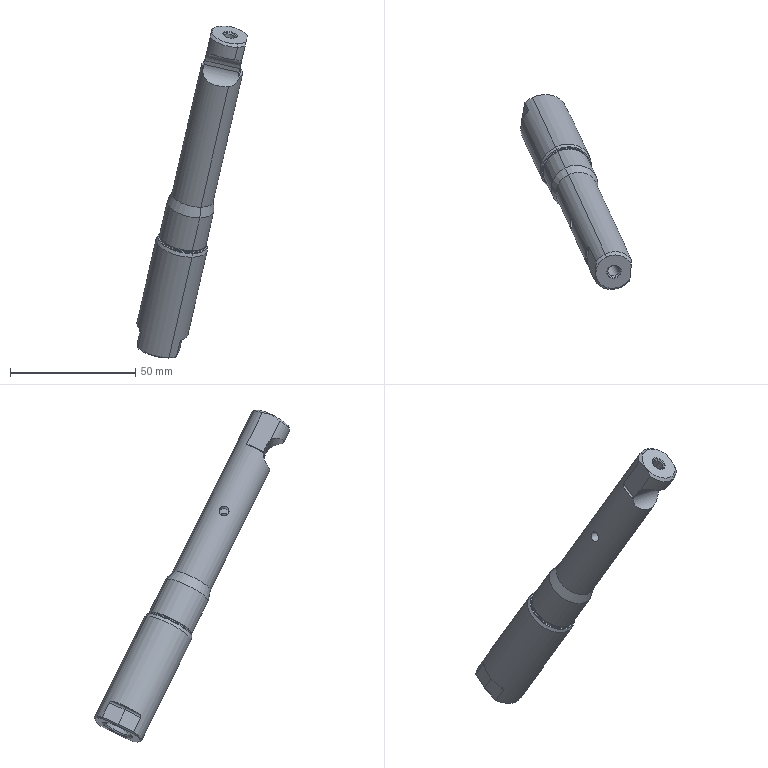Part | SolidWorks | features BaseBody 1 | 1 solid | 77 faces | box 44.117 x 78.054 x 132.466 mm | volume 28853 mm3 | cylinder 30 | cone 25 | plane 18 | torus 4 | commonest cylinder face diameters 2 x4 3.983 x4 16.8 x4 1 x2 4.5 x2 8.665 x2